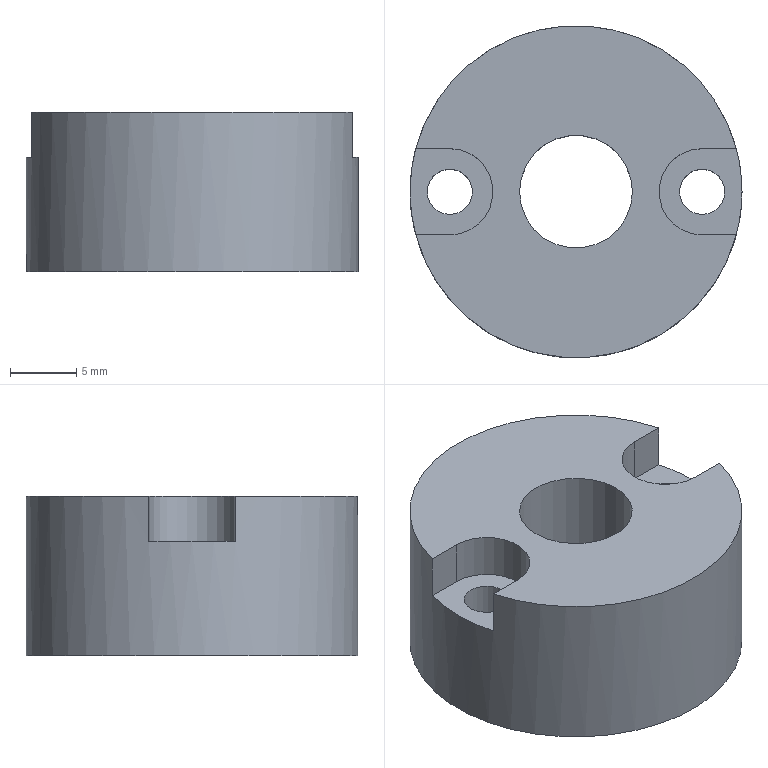Part | NX | features BREP 1 | 1 solid | 18 faces | box 25 x 25 x 12 mm | volume 4603 mm3 | plane 8 | cylinder 8 | cone 2 | commonest cylinder face diameters 3.4 x2 4 x2 6.5 x2 8.5 x1 25 x1
STEP:
#1=CARTESIAN_POINT('',(4.25,0.,12.));
#2=VERTEX_POINT('',#1);
#3=CARTESIAN_POINT('',(0.,0.,12.));
#4=DIRECTION('',(0.,0.,1.));
#5=DIRECTION('',(1.,0.,0.));
#6=AXIS2_PLACEMENT_3D('',#3,#4,#5);
#7=CIRCLE('',#6,4.25);
#8=EDGE_CURVE('',#2,#2,#7,.T.);
#9=ORIENTED_EDGE('',*,*,#8,.F.);
#10=EDGE_LOOP('',(#9));
#11=FACE_BOUND('',#10,.T.);
#12=CARTESIAN_POINT('',(-9.5,-3.25,12.));
#13=VERTEX_POINT('',#12);
#14=CARTESIAN_POINT('',(-9.5,3.25,12.));
#15=VERTEX_POINT('',#14);
#16=CARTESIAN_POINT('',(-9.5,0.,12.));
#17=DIRECTION('',(0.,0.,1.));
#18=DIRECTION('',(1.,0.,0.));
#19=AXIS2_PLACEMENT_3D('',#16,#17,#18);
#20=CIRCLE('',#19,3.25);
#21=EDGE_CURVE('',#13,#15,#20,.T.);
#22=ORIENTED_EDGE('',*,*,#21,.F.);
#23=CARTESIAN_POINT('',(-12.07,-3.25,12.));
#24=VERTEX_POINT('',#23);
#25=CARTESIAN_POINT('',(-9.5,-3.25,12.));
#26=DIRECTION('',(-1.,0.,0.));
#27=VECTOR('',#26,1000.);
#28=LINE('',#25,#27);
#29=EDGE_CURVE('',#13,#24,#28,.T.);
#30=ORIENTED_EDGE('',*,*,#29,.T.);
#31=CARTESIAN_POINT('',(12.07,-3.25,12.));
#32=VERTEX_POINT('',#31);
#33=CARTESIAN_POINT('',(0.,0.,12.));
#34=DIRECTION('',(0.,0.,1.));
#35=DIRECTION('',(1.,0.,0.));
#36=AXIS2_PLACEMENT_3D('',#33,#34,#35);
#37=CIRCLE('',#36,12.5);
#38=EDGE_CURVE('',#24,#32,#37,.T.);
#39=ORIENTED_EDGE('',*,*,#38,.T.);
#40=CARTESIAN_POINT('',(9.5,-3.25,12.));
#41=VERTEX_POINT('',#40);
#42=CARTESIAN_POINT('',(9.5,-3.25,12.));
#43=DIRECTION('',(1.,0.,0.));
#44=VECTOR('',#43,1000.);
#45=LINE('',#42,#44);
#46=EDGE_CURVE('',#41,#32,#45,.T.);
#47=ORIENTED_EDGE('',*,*,#46,.F.);
#48=CARTESIAN_POINT('',(9.5,3.25,12.));
#49=VERTEX_POINT('',#48);
#50=CARTESIAN_POINT('',(9.5,0.,12.));
#51=DIRECTION('',(0.,0.,1.));
#52=DIRECTION('',(1.,0.,0.));
#53=AXIS2_PLACEMENT_3D('',#50,#51,#52);
#54=CIRCLE('',#53,3.25);
#55=EDGE_CURVE('',#49,#41,#54,.T.);
#56=ORIENTED_EDGE('',*,*,#55,.F.);
#57=CARTESIAN_POINT('',(12.07,3.25,12.));
#58=VERTEX_POINT('',#57);
#59=CARTESIAN_POINT('',(12.5,3.25,12.));
#60=DIRECTION('',(-1.,0.,0.));
#61=VECTOR('',#60,1000.);
#62=LINE('',#59,#61);
#63=EDGE_CURVE('',#58,#49,#62,.T.);
#64=ORIENTED_EDGE('',*,*,#63,.F.);
#65=CARTESIAN_POINT('',(-12.07,3.25,12.));
#66=VERTEX_POINT('',#65);
#67=CARTESIAN_POINT('',(0.,0.,12.));
#68=DIRECTION('',(0.,0.,1.));
#69=DIRECTION('',(1.,0.,0.));
#70=AXIS2_PLACEMENT_3D('',#67,#68,#69);
#71=CIRCLE('',#70,12.5);
#72=EDGE_CURVE('',#58,#66,#71,.T.);
#73=ORIENTED_EDGE('',*,*,#72,.T.);
#74=CARTESIAN_POINT('',(-12.5,3.25,12.));
#75=DIRECTION('',(1.,0.,0.));
#76=VECTOR('',#75,1000.);
#77=LINE('',#74,#76);
#78=EDGE_CURVE('',#66,#15,#77,.T.);
#79=ORIENTED_EDGE('',*,*,#78,.T.);
#80=EDGE_LOOP('',(#22,#30,#39,#47,#56,#64,#73,#79));
#81=FACE_BOUND('',#80,.T.);
#82=CARTESIAN_POINT('',(0.,0.,12.));
#83=DIRECTION('',(0.,0.,1.));
#84=DIRECTION('',(-1.,0.,0.));
#85=AXIS2_PLACEMENT_3D('',#82,#83,#84);
#86=PLANE('',#85);
#87=ADVANCED_FACE('',(#11,#81),#86,.T.);
#88=CARTESIAN_POINT('',(12.5,0.,0.));
#89=VERTEX_POINT('',#88);
#90=CARTESIAN_POINT('',(0.,0.,0.));
#91=DIRECTION('',(0.,0.,1.));
#92=DIRECTION('',(1.,0.,0.));
#93=AXIS2_PLACEMENT_3D('',#90,#91,#92);
#94=CIRCLE('',#93,12.5);
#95=EDGE_CURVE('',#89,#89,#94,.T.);
#96=ORIENTED_EDGE('',*,*,#95,.T.);
#97=EDGE_LOOP('',(#96));
#98=FACE_BOUND('',#97,.T.);
#99=CARTESIAN_POINT('',(-12.07,3.25,8.6));
#100=VERTEX_POINT('',#99);
#101=CARTESIAN_POINT('',(-12.07,3.25,12.));
#102=DIRECTION('',(0.,0.,-1.));
#103=VECTOR('',#102,1000.);
#104=LINE('',#101,#103);
#105=EDGE_CURVE('',#66,#100,#104,.T.);
#106=ORIENTED_EDGE('',*,*,#105,.F.);
#107=ORIENTED_EDGE('',*,*,#72,.F.);
#108=CARTESIAN_POINT('',(12.07,3.25,8.6));
#109=VERTEX_POINT('',#108);
#110=CARTESIAN_POINT('',(12.07,3.25,12.));
#111=DIRECTION('',(0.,0.,-1.));
#112=VECTOR('',#111,1000.);
#113=LINE('',#110,#112);
#114=EDGE_CURVE('',#58,#109,#113,.T.);
#115=ORIENTED_EDGE('',*,*,#114,.T.);
#116=CARTESIAN_POINT('',(12.07,-3.25,8.6));
#117=VERTEX_POINT('',#116);
#118=CARTESIAN_POINT('',(0.,0.,8.6));
#119=DIRECTION('',(0.,0.,-1.));
#120=DIRECTION('',(-1.,0.,0.));
#121=AXIS2_PLACEMENT_3D('',#118,#119,#120);
#122=CIRCLE('',#121,12.5);
#123=EDGE_CURVE('',#109,#117,#122,.T.);
#124=ORIENTED_EDGE('',*,*,#123,.T.);
#125=CARTESIAN_POINT('',(12.07,-3.25,12.));
#126=DIRECTION('',(0.,0.,1.));
#127=VECTOR('',#126,1000.);
#128=LINE('',#125,#127);
#129=EDGE_CURVE('',#117,#32,#128,.T.);
#130=ORIENTED_EDGE('',*,*,#129,.T.);
#131=ORIENTED_EDGE('',*,*,#38,.F.);
#132=CARTESIAN_POINT('',(-12.07,-3.25,8.6));
#133=VERTEX_POINT('',#132);
#134=CARTESIAN_POINT('',(-12.07,-3.25,12.));
#135=DIRECTION('',(0.,0.,1.));
#136=VECTOR('',#135,1000.);
#137=LINE('',#134,#136);
#138=EDGE_CURVE('',#133,#24,#137,.T.);
#139=ORIENTED_EDGE('',*,*,#138,.F.);
#140=CARTESIAN_POINT('',(0.,0.,8.6));
#141=DIRECTION('',(0.,0.,-1.));
#142=DIRECTION('',(-1.,0.,0.));
#143=AXIS2_PLACEMENT_3D('',#140,#141,#142);
#144=CIRCLE('',#143,12.5);
#145=EDGE_CURVE('',#133,#100,#144,.T.);
#146=ORIENTED_EDGE('',*,*,#145,.T.);
#147=EDGE_LOOP('',(#106,#107,#115,#124,#130,#131,#139,#146));
#148=FACE_BOUND('',#147,.T.);
#149=CARTESIAN_POINT('',(0.,0.,12.));
#150=DIRECTION('',(0.,0.,-1.));
#151=DIRECTION('',(1.,0.,0.));
#152=AXIS2_PLACEMENT_3D('',#149,#150,#151);
#153=CYLINDRICAL_SURFACE('',#152,12.5);
#154=ADVANCED_FACE('',(#98,#148),#153,.T.);
#155=CARTESIAN_POINT('',(-9.5,-3.25,8.6));
#156=VERTEX_POINT('',#155);
#157=CARTESIAN_POINT('',(-9.5,-3.25,8.6));
#158=DIRECTION('',(0.,0.,1.));
#159=VECTOR('',#158,1000.);
#160=LINE('',#157,#159);
#161=EDGE_CURVE('',#156,#13,#160,.T.);
#162=ORIENTED_EDGE('',*,*,#161,.T.);
#163=ORIENTED_EDGE('',*,*,#21,.T.);
#164=CARTESIAN_POINT('',(-9.5,3.25,8.6));
#165=VERTEX_POINT('',#164);
#166=CARTESIAN_POINT('',(-9.5,3.25,8.6));
#167=DIRECTION('',(0.,0.,1.));
#168=VECTOR('',#167,1000.);
#169=LINE('',#166,#168);
#170=EDGE_CURVE('',#165,#15,#169,.T.);
#171=ORIENTED_EDGE('',*,*,#170,.F.);
#172=CARTESIAN_POINT('',(-9.5,0.,8.6));
#173=DIRECTION('',(0.,0.,1.));
#174=DIRECTION('',(1.,0.,0.));
#175=AXIS2_PLACEMENT_3D('',#172,#173,#174);
#176=CIRCLE('',#175,3.25);
#177=EDGE_CURVE('',#156,#165,#176,.T.);
#178=ORIENTED_EDGE('',*,*,#177,.F.);
#179=EDGE_LOOP('',(#162,#163,#171,#178));
#180=FACE_BOUND('',#179,.T.);
#181=CARTESIAN_POINT('',(-9.5,0.,12.));
#182=DIRECTION('',(0.,0.,1.));
#183=DIRECTION('',(-1.,0.,0.));
#184=AXIS2_PLACEMENT_3D('',#181,#182,#183);
#185=CYLINDRICAL_SURFACE('',#184,3.25);
#186=ADVANCED_FACE('',(#180),#185,.F.);
#187=CARTESIAN_POINT('',(9.5,3.25,8.6));
#188=VERTEX_POINT('',#187);
#189=CARTESIAN_POINT('',(9.5,3.25,8.6));
#190=DIRECTION('',(0.,0.,1.));
#191=VECTOR('',#190,1000.);
#192=LINE('',#189,#191);
#193=EDGE_CURVE('',#188,#49,#192,.T.);
#194=ORIENTED_EDGE('',*,*,#193,.T.);
#195=ORIENTED_EDGE('',*,*,#55,.T.);
#196=CARTESIAN_POINT('',(9.5,-3.25,8.6));
#197=VERTEX_POINT('',#196);
#198=CARTESIAN_POINT('',(9.5,-3.25,8.6));
#199=DIRECTION('',(0.,0.,1.));
#200=VECTOR('',#199,1000.);
#201=LINE('',#198,#200);
#202=EDGE_CURVE('',#197,#41,#201,.T.);
#203=ORIENTED_EDGE('',*,*,#202,.F.);
#204=CARTESIAN_POINT('',(9.5,0.,8.6));
#205=DIRECTION('',(0.,0.,1.));
#206=DIRECTION('',(1.,0.,0.));
#207=AXIS2_PLACEMENT_3D('',#204,#205,#206);
#208=CIRCLE('',#207,3.25);
#209=EDGE_CURVE('',#188,#197,#208,.T.);
#210=ORIENTED_EDGE('',*,*,#209,.F.);
#211=EDGE_LOOP('',(#194,#195,#203,#210));
#212=FACE_BOUND('',#211,.T.);
#213=CARTESIAN_POINT('',(9.5,0.,12.));
#214=DIRECTION('',(0.,0.,1.));
#215=DIRECTION('',(-1.,0.,0.));
#216=AXIS2_PLACEMENT_3D('',#213,#214,#215);
#217=CYLINDRICAL_SURFACE('',#216,3.25);
#218=ADVANCED_FACE('',(#212),#217,.F.);
#219=CARTESIAN_POINT('',(11.2,0.,0.));
#220=VERTEX_POINT('',#219);
#221=CARTESIAN_POINT('',(9.5,0.,0.));
#222=DIRECTION('',(0.,0.,1.));
#223=DIRECTION('',(1.,0.,0.));
#224=AXIS2_PLACEMENT_3D('',#221,#222,#223);
#225=CIRCLE('',#224,1.7);
#226=EDGE_CURVE('',#220,#220,#225,.T.);
#227=ORIENTED_EDGE('',*,*,#226,.T.);
#228=EDGE_LOOP('',(#227));
#229=FACE_BOUND('',#228,.T.);
#230=CARTESIAN_POINT('',(-7.8,0.,0.));
#231=VERTEX_POINT('',#230);
#232=CARTESIAN_POINT('',(-9.5,0.,0.));
#233=DIRECTION('',(0.,0.,1.));
#234=DIRECTION('',(1.,0.,0.));
#235=AXIS2_PLACEMENT_3D('',#232,#233,#234);
#236=CIRCLE('',#235,1.7);
#237=EDGE_CURVE('',#231,#231,#236,.T.);
#238=ORIENTED_EDGE('',*,*,#237,.T.);
#239=EDGE_LOOP('',(#238));
#240=FACE_BOUND('',#239,.T.);
#241=CARTESIAN_POINT('',(-2.,-9.5,0.));
#242=VERTEX_POINT('',#241);
#243=CARTESIAN_POINT('',(0.,-9.5,0.));
#244=DIRECTION('',(0.,0.,-1.));
#245=DIRECTION('',(-1.,0.,0.));
#246=AXIS2_PLACEMENT_3D('',#243,#244,#245);
#247=CIRCLE('',#246,2.);
#248=EDGE_CURVE('',#242,#242,#247,.T.);
#249=ORIENTED_EDGE('',*,*,#248,.F.);
#250=EDGE_LOOP('',(#249));
#251=FACE_BOUND('',#250,.T.);
#252=CARTESIAN_POINT('',(-2.,9.5,0.));
#253=VERTEX_POINT('',#252);
#254=CARTESIAN_POINT('',(0.,9.5,0.));
#255=DIRECTION('',(0.,0.,-1.));
#256=DIRECTION('',(-1.,0.,0.));
#257=AXIS2_PLACEMENT_3D('',#254,#255,#256);
#258=CIRCLE('',#257,2.);
#259=EDGE_CURVE('',#253,#253,#258,.T.);
#260=ORIENTED_EDGE('',*,*,#259,.F.);
#261=EDGE_LOOP('',(#260));
#262=FACE_BOUND('',#261,.T.);
#263=ORIENTED_EDGE('',*,*,#95,.F.);
#264=EDGE_LOOP('',(#263));
#265=FACE_BOUND('',#264,.T.);
#266=CARTESIAN_POINT('',(4.25,0.,0.));
#267=VERTEX_POINT('',#266);
#268=CARTESIAN_POINT('',(0.,0.,0.));
#269=DIRECTION('',(0.,0.,1.));
#270=DIRECTION('',(1.,0.,0.));
#271=AXIS2_PLACEMENT_3D('',#268,#269,#270);
#272=CIRCLE('',#271,4.25);
#273=EDGE_CURVE('',#267,#267,#272,.T.);
#274=ORIENTED_EDGE('',*,*,#273,.T.);
#275=EDGE_LOOP('',(#274));
#276=FACE_BOUND('',#275,.T.);
#277=CARTESIAN_POINT('',(0.,0.,0.));
#278=DIRECTION('',(0.,0.,1.));
#279=DIRECTION('',(-1.,0.,0.));
#280=AXIS2_PLACEMENT_3D('',#277,#278,#279);
#281=PLANE('',#280);
#282=ADVANCED_FACE('',(#229,#240,#251,#262,#265,#276),#281,.F.);
#283=ORIENTED_EDGE('',*,*,#8,.T.);
#284=EDGE_LOOP('',(#283));
#285=FACE_BOUND('',#284,.T.);
#286=ORIENTED_EDGE('',*,*,#273,.F.);
#287=EDGE_LOOP('',(#286));
#288=FACE_BOUND('',#287,.T.);
#289=CARTESIAN_POINT('',(0.,0.,12.));
#290=DIRECTION('',(0.,0.,-1.));
#291=DIRECTION('',(1.,0.,0.));
#292=AXIS2_PLACEMENT_3D('',#289,#290,#291);
#293=CYLINDRICAL_SURFACE('',#292,4.25);
#294=ADVANCED_FACE('',(#285,#288),#293,.F.);
#295=CARTESIAN_POINT('',(0.,9.5,9.202));
#296=VERTEX_POINT('',#295);
#297=VERTEX_LOOP('',#296);
#298=FACE_BOUND('',#297,.T.);
#299=CARTESIAN_POINT('',(-2.,9.5,8.));
#300=VERTEX_POINT('',#299);
#301=CARTESIAN_POINT('',(0.,9.5,8.));
#302=DIRECTION('',(0.,0.,-1.));
#303=DIRECTION('',(-1.,0.,0.));
#304=AXIS2_PLACEMENT_3D('',#301,#302,#303);
#305=CIRCLE('',#304,2.);
#306=EDGE_CURVE('',#300,#300,#305,.T.);
#307=ORIENTED_EDGE('',*,*,#306,.T.);
#308=EDGE_LOOP('',(#307));
#309=FACE_BOUND('',#308,.T.);
#310=CARTESIAN_POINT('',(0.,9.5,8.));
#311=DIRECTION('',(0.,0.,-1.));
#312=DIRECTION('',(1.,0.,0.));
#313=AXIS2_PLACEMENT_3D('',#310,#311,#312);
#314=CONICAL_SURFACE('',#313,2.,1.03);
#315=ADVANCED_FACE('',(#298,#309),#314,.F.);
#316=ORIENTED_EDGE('',*,*,#306,.F.);
#317=EDGE_LOOP('',(#316));
#318=FACE_BOUND('',#317,.T.);
#319=ORIENTED_EDGE('',*,*,#259,.T.);
#320=EDGE_LOOP('',(#319));
#321=FACE_BOUND('',#320,.T.);
#322=CARTESIAN_POINT('',(0.,9.5,0.));
#323=DIRECTION('',(0.,0.,-1.));
#324=DIRECTION('',(1.,0.,0.));
#325=AXIS2_PLACEMENT_3D('',#322,#323,#324);
#326=CYLINDRICAL_SURFACE('',#325,2.);
#327=ADVANCED_FACE('',(#318,#321),#326,.F.);
#328=CARTESIAN_POINT('',(0.,-9.5,9.202));
#329=VERTEX_POINT('',#328);
#330=VERTEX_LOOP('',#329);
#331=FACE_BOUND('',#330,.T.);
#332=CARTESIAN_POINT('',(-2.,-9.5,8.));
#333=VERTEX_POINT('',#332);
#334=CARTESIAN_POINT('',(0.,-9.5,8.));
#335=DIRECTION('',(0.,0.,-1.));
#336=DIRECTION('',(-1.,0.,0.));
#337=AXIS2_PLACEMENT_3D('',#334,#335,#336);
#338=CIRCLE('',#337,2.);
#339=EDGE_CURVE('',#333,#333,#338,.T.);
#340=ORIENTED_EDGE('',*,*,#339,.T.);
#341=EDGE_LOOP('',(#340));
#342=FACE_BOUND('',#341,.T.);
#343=CARTESIAN_POINT('',(0.,-9.5,8.));
#344=DIRECTION('',(0.,0.,-1.));
#345=DIRECTION('',(1.,0.,0.));
#346=AXIS2_PLACEMENT_3D('',#343,#344,#345);
#347=CONICAL_SURFACE('',#346,2.,1.03);
#348=ADVANCED_FACE('',(#331,#342),#347,.F.);
#349=ORIENTED_EDGE('',*,*,#339,.F.);
#350=EDGE_LOOP('',(#349));
#351=FACE_BOUND('',#350,.T.);
#352=ORIENTED_EDGE('',*,*,#248,.T.);
#353=EDGE_LOOP('',(#352));
#354=FACE_BOUND('',#353,.T.);
#355=CARTESIAN_POINT('',(0.,-9.5,0.));
#356=DIRECTION('',(0.,0.,-1.));
#357=DIRECTION('',(1.,0.,0.));
#358=AXIS2_PLACEMENT_3D('',#355,#356,#357);
#359=CYLINDRICAL_SURFACE('',#358,2.);
#360=ADVANCED_FACE('',(#351,#354),#359,.F.);
#361=CARTESIAN_POINT('',(-7.8,0.,8.6));
#362=VERTEX_POINT('',#361);
#363=CARTESIAN_POINT('',(-9.5,0.,8.6));
#364=DIRECTION('',(0.,0.,1.));
#365=DIRECTION('',(1.,0.,0.));
#366=AXIS2_PLACEMENT_3D('',#363,#364,#365);
#367=CIRCLE('',#366,1.7);
#368=EDGE_CURVE('',#362,#362,#367,.T.);
#369=ORIENTED_EDGE('',*,*,#368,.F.);
#370=EDGE_LOOP('',(#369));
#371=FACE_BOUND('',#370,.T.);
#372=ORIENTED_EDGE('',*,*,#145,.F.);
#373=CARTESIAN_POINT('',(-9.5,-3.25,8.6));
#374=DIRECTION('',(-1.,0.,0.));
#375=VECTOR('',#374,1000.);
#376=LINE('',#373,#375);
#377=EDGE_CURVE('',#156,#133,#376,.T.);
#378=ORIENTED_EDGE('',*,*,#377,.F.);
#379=ORIENTED_EDGE('',*,*,#177,.T.);
#380=CARTESIAN_POINT('',(-12.5,3.25,8.6));
#381=DIRECTION('',(1.,0.,0.));
#382=VECTOR('',#381,1000.);
#383=LINE('',#380,#382);
#384=EDGE_CURVE('',#100,#165,#383,.T.);
#385=ORIENTED_EDGE('',*,*,#384,.F.);
#386=EDGE_LOOP('',(#372,#378,#379,#385));
#387=FACE_BOUND('',#386,.T.);
#388=CARTESIAN_POINT('',(-7.8,0.,8.6));
#389=DIRECTION('',(0.,0.,-1.));
#390=DIRECTION('',(1.,0.,0.));
#391=AXIS2_PLACEMENT_3D('',#388,#389,#390);
#392=PLANE('',#391);
#393=ADVANCED_FACE('',(#371,#387),#392,.F.);
#394=ORIENTED_EDGE('',*,*,#237,.F.);
#395=EDGE_LOOP('',(#394));
#396=FACE_BOUND('',#395,.T.);
#397=ORIENTED_EDGE('',*,*,#368,.T.);
#398=EDGE_LOOP('',(#397));
#399=FACE_BOUND('',#398,.T.);
#400=CARTESIAN_POINT('',(-9.5,0.,12.));
#401=DIRECTION('',(0.,0.,1.));
#402=DIRECTION('',(-1.,0.,0.));
#403=AXIS2_PLACEMENT_3D('',#400,#401,#402);
#404=CYLINDRICAL_SURFACE('',#403,1.7);
#405=ADVANCED_FACE('',(#396,#399),#404,.F.);
#406=CARTESIAN_POINT('',(11.2,0.,8.6));
#407=VERTEX_POINT('',#406);
#408=CARTESIAN_POINT('',(9.5,0.,8.6));
#409=DIRECTION('',(0.,0.,1.));
#410=DIRECTION('',(1.,0.,0.));
#411=AXIS2_PLACEMENT_3D('',#408,#409,#410);
#412=CIRCLE('',#411,1.7);
#413=EDGE_CURVE('',#407,#407,#412,.T.);
#414=ORIENTED_EDGE('',*,*,#413,.F.);
#415=EDGE_LOOP('',(#414));
#416=FACE_BOUND('',#415,.T.);
#417=ORIENTED_EDGE('',*,*,#209,.T.);
#418=CARTESIAN_POINT('',(9.5,-3.25,8.6));
#419=DIRECTION('',(1.,0.,0.));
#420=VECTOR('',#419,1000.);
#421=LINE('',#418,#420);
#422=EDGE_CURVE('',#197,#117,#421,.T.);
#423=ORIENTED_EDGE('',*,*,#422,.T.);
#424=ORIENTED_EDGE('',*,*,#123,.F.);
#425=CARTESIAN_POINT('',(12.5,3.25,8.6));
#426=DIRECTION('',(-1.,0.,0.));
#427=VECTOR('',#426,1000.);
#428=LINE('',#425,#427);
#429=EDGE_CURVE('',#109,#188,#428,.T.);
#430=ORIENTED_EDGE('',*,*,#429,.T.);
#431=EDGE_LOOP('',(#417,#423,#424,#430));
#432=FACE_BOUND('',#431,.T.);
#433=CARTESIAN_POINT('',(11.2,0.,8.6));
#434=DIRECTION('',(0.,0.,-1.));
#435=DIRECTION('',(1.,0.,0.));
#436=AXIS2_PLACEMENT_3D('',#433,#434,#435);
#437=PLANE('',#436);
#438=ADVANCED_FACE('',(#416,#432),#437,.F.);
#439=ORIENTED_EDGE('',*,*,#226,.F.);
#440=EDGE_LOOP('',(#439));
#441=FACE_BOUND('',#440,.T.);
#442=ORIENTED_EDGE('',*,*,#413,.T.);
#443=EDGE_LOOP('',(#442));
#444=FACE_BOUND('',#443,.T.);
#445=CARTESIAN_POINT('',(9.5,0.,12.));
#446=DIRECTION('',(0.,0.,1.));
#447=DIRECTION('',(-1.,0.,0.));
#448=AXIS2_PLACEMENT_3D('',#445,#446,#447);
#449=CYLINDRICAL_SURFACE('',#448,1.7);
#450=ADVANCED_FACE('',(#441,#444),#449,.F.);
#451=ORIENTED_EDGE('',*,*,#63,.T.);
#452=ORIENTED_EDGE('',*,*,#193,.F.);
#453=ORIENTED_EDGE('',*,*,#429,.F.);
#454=ORIENTED_EDGE('',*,*,#114,.F.);
#455=EDGE_LOOP('',(#451,#452,#453,#454));
#456=FACE_BOUND('',#455,.T.);
#457=CARTESIAN_POINT('',(12.5,3.25,8.6));
#458=DIRECTION('',(0.,1.,0.));
#459=DIRECTION('',(0.,0.,-1.));
#460=AXIS2_PLACEMENT_3D('',#457,#458,#459);
#461=PLANE('',#460);
#462=ADVANCED_FACE('',(#456),#461,.F.);
#463=ORIENTED_EDGE('',*,*,#422,.F.);
#464=ORIENTED_EDGE('',*,*,#202,.T.);
#465=ORIENTED_EDGE('',*,*,#46,.T.);
#466=ORIENTED_EDGE('',*,*,#129,.F.);
#467=EDGE_LOOP('',(#463,#464,#465,#466));
#468=FACE_BOUND('',#467,.T.);
#469=CARTESIAN_POINT('',(9.5,-3.25,8.6));
#470=DIRECTION('',(0.,-1.,0.));
#471=DIRECTION('',(0.,0.,1.));
#472=AXIS2_PLACEMENT_3D('',#469,#470,#471);
#473=PLANE('',#472);
#474=ADVANCED_FACE('',(#468),#473,.F.);
#475=ORIENTED_EDGE('',*,*,#105,.T.);
#476=ORIENTED_EDGE('',*,*,#384,.T.);
#477=ORIENTED_EDGE('',*,*,#170,.T.);
#478=ORIENTED_EDGE('',*,*,#78,.F.);
#479=EDGE_LOOP('',(#475,#476,#477,#478));
#480=FACE_BOUND('',#479,.T.);
#481=CARTESIAN_POINT('',(-12.5,3.25,8.6));
#482=DIRECTION('',(0.,-1.,0.));
#483=DIRECTION('',(0.,0.,1.));
#484=AXIS2_PLACEMENT_3D('',#481,#482,#483);
#485=PLANE('',#484);
#486=ADVANCED_FACE('',(#480),#485,.T.);
#487=ORIENTED_EDGE('',*,*,#138,.T.);
#488=ORIENTED_EDGE('',*,*,#29,.F.);
#489=ORIENTED_EDGE('',*,*,#161,.F.);
#490=ORIENTED_EDGE('',*,*,#377,.T.);
#491=EDGE_LOOP('',(#487,#488,#489,#490));
#492=FACE_BOUND('',#491,.T.);
#493=CARTESIAN_POINT('',(-9.5,-3.25,8.6));
#494=DIRECTION('',(0.,1.,0.));
#495=DIRECTION('',(0.,0.,-1.));
#496=AXIS2_PLACEMENT_3D('',#493,#494,#495);
#497=PLANE('',#496);
#498=ADVANCED_FACE('',(#492),#497,.T.);
#499=CLOSED_SHELL('',(#87,#154,#186,#218,#282,#294,#315,#327,#348,#360,#393,#405,#438,#450,#462,#474,#486,#498));
#500=MANIFOLD_SOLID_BREP('',#499);
#501=(LENGTH_UNIT()NAMED_UNIT(*)SI_UNIT(.MILLI.,.METRE.));
#502=UNCERTAINTY_MEASURE_WITH_UNIT(LENGTH_MEASURE(0.00001),#501,'','');
#503=(NAMED_UNIT(*)PLANE_ANGLE_UNIT()SI_UNIT($,.RADIAN.));
#504=(NAMED_UNIT(*)SI_UNIT($,.STERADIAN.)SOLID_ANGLE_UNIT());
#505=(GEOMETRIC_REPRESENTATION_CONTEXT(3)GLOBAL_UNCERTAINTY_ASSIGNED_CONTEXT((#502))GLOBAL_UNIT_ASSIGNED_CONTEXT((#501,#503,#504))REPRESENTATION_CONTEXT('',''));
#506=ADVANCED_BREP_SHAPE_REPRESENTATION('',(#500),#505);